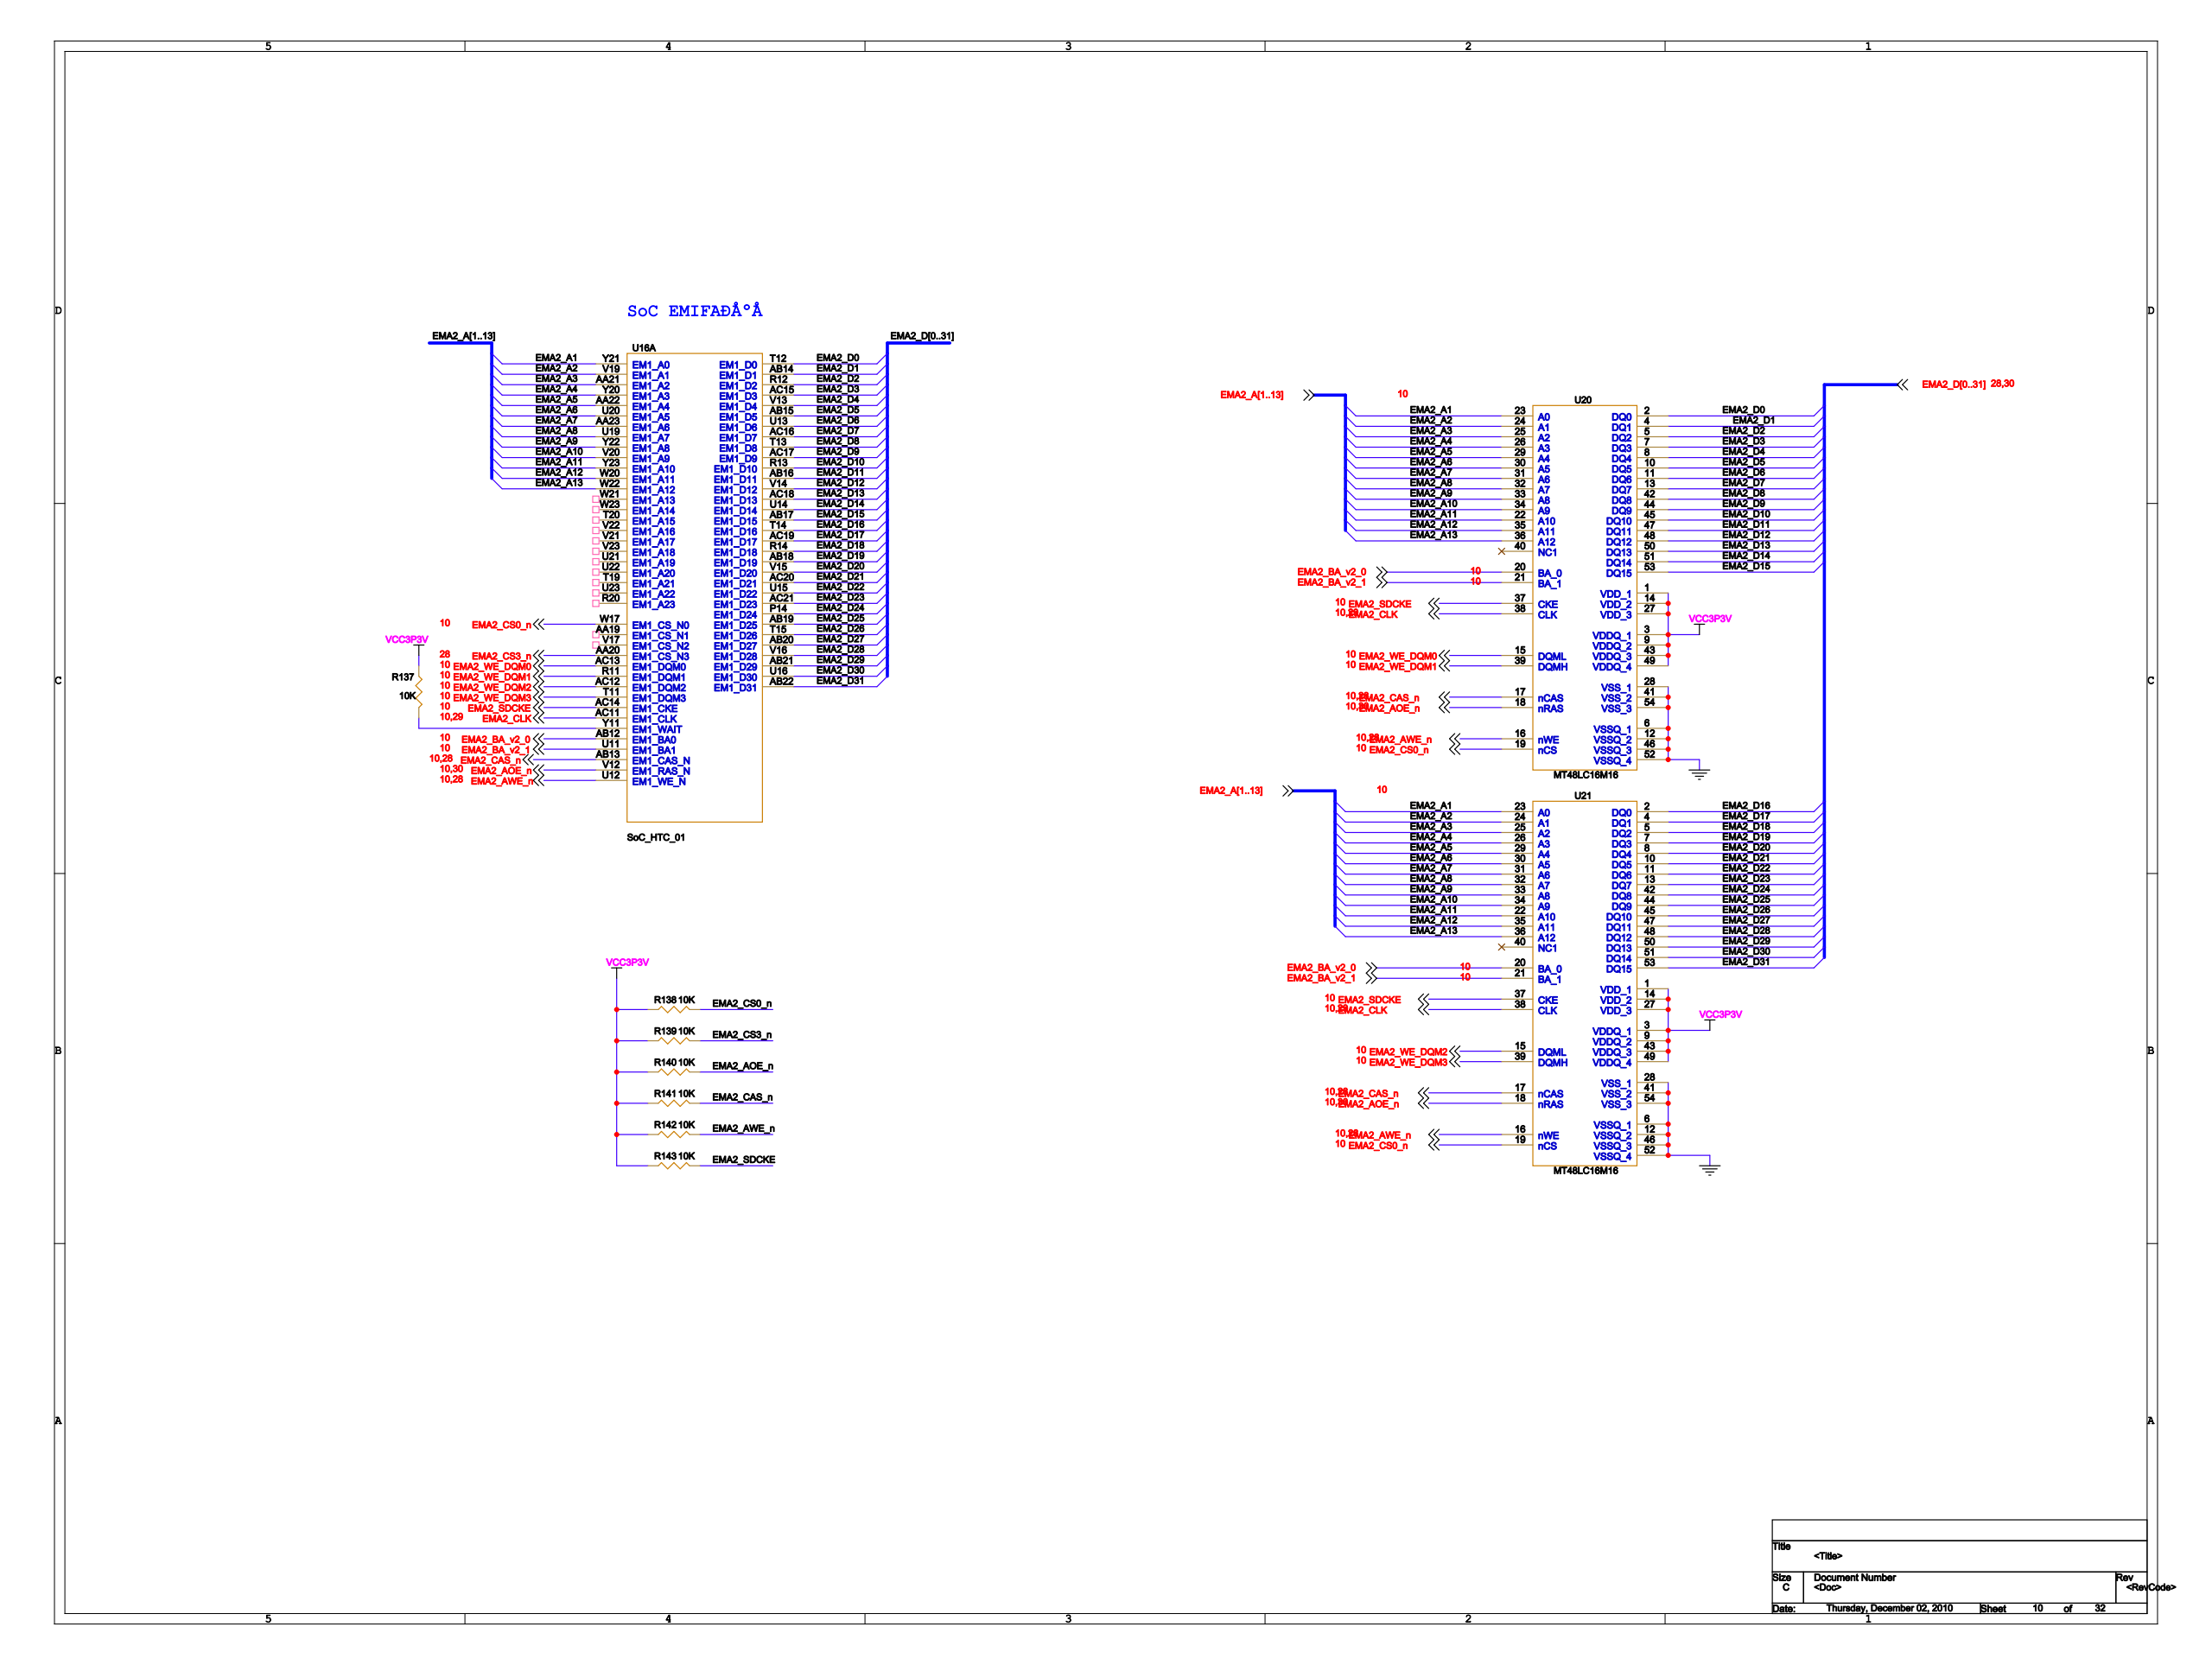Circuit board | Cadence Allegro | 1001 parts | 1318 nets | one sheet of the schematic
Parts on this sheet (reference | value | footprint):
R137 | 10K | 0603
R138 | 10K | 0603
R139 | 10K | 0603
R140 | 10K | 0603
R141 | 10K | 0603
R142 | 10K | 0603
R143 | 10K | 0603
U11 | MT48LC32M16 | TSOP54
U14 | MT48LC16M16 | TSOP54
U15 | MT48LC16M16 | TSOP54
U16 | SoC_HTC_01 | L529_XIN
U20 | MT48LC16M16 | TSOP54
U21 | MT48LC16M16 | TSOP54
U23 | MT48LC32M16 | TSOP54
Nets of these parts (net: part-pin ...):
EMA2_D11: U16-AB16 U20-47
EMA2_D3: U16-AC15 U20-7
EMA2_D7: U16-AC16 U20-13
EMA2_D15: U16-AB17 U20-53
EMA2_D27: U16-AB20 U21-47
EMA2_D23: U16-AC21 U21-13
EMA2_D29: U16-AB21 U21-50
EMA2_D31: U16-AB22 U21-53
EMA2_D9: U16-AC17 U20-44
EMA2_D12: U16-V14 U20-48
EMA2_AOE_N: R140-2 U16-V12 U20-18 U21-18
EMA2_D17: U16-AC19 U21-4
EMA2_D13: U16-AC18 U20-50
EMA2_D25: U16-AB19 U21-44
EMA2_D4: U16-V13 U20-8
EMA2_AWE_N: R142-2 U16-U12 U20-16 U21-16
EMA2_D6: U16-U13 U20-11
EMA2_CAS_N: R141-2 U16-AB13 U20-17 U21-17
EMA2_D5: U16-AB15 U20-10
EMA2_D22: U16-U15 U21-11
EMA2_D28: U16-V16 U21-48
EMA2_D21: U16-AC20 U21-10
EMA2_D1: U16-AB14 U20-4
EMA2_D2: U16-R12 U20-5
EMA2_D20: U16-V15 U21-8
EMA2_CS3_N: R139-2 U16-AA20
EMA2_D0: U16-T12 U20-2
EMA2_D30: U16-U16 U21-51
EMA2_D8: U16-T13 U20-42
EMA2_CLK: U16-AC11 U20-38 U21-38
EMA2_D10: U16-R13 U20-45
EMA2_D24: U16-P14 U21-42
EMA2_D16: U16-T14 U21-2
EMA2_D14: U16-U14 U20-51
EMA2_D26: U16-T15 U21-45
EMA2_D18: U16-R14 U21-5
EMA2_D19: U16-AB18 U21-7
VCC3P3V: R137-2 R138-1 R139-1 R140-1 R141-1 R142-1 R143-1 U11-1 U11-3 U11-9 U11-14 U11-27 U11-43 U11-49 U14-1 U14-3 U14-9 U14-14 U14-27 U14-43 U14-49 U15-1 U15-3 U15-9 U15-14 U15-27 U15-43 U15-49 U20-1 U20-3 U20-9 U20-14 U20-27 U20-43 U20-49 U21-1 U21-3 U21-9 U21-14 U21-27 U21-43 U21-49 U23-1 U23-3 U23-9 U23-14 U23-27 U23-43 U23-49
EMA2_A1: U16-Y21 U20-23 U21-23
EMA2_A2: U16-V19 U20-24 U21-24
EMA2_A11: U16-Y23 U20-22 U21-22
EMA2_A12: U16-W20 U20-35 U21-35
EMA2_A13: U16-W22 U20-36 U21-36
EMA2_A3: U16-AA21 U20-25 U21-25
EMA2_A4: U16-Y20 U20-26 U21-26
EMA2_A5: U16-AA22 U20-29 U21-29
EMA2_A6: U16-U20 U20-30 U21-30
EMA2_A7: U16-AA23 U20-31 U21-31
EMA2_A8: U16-U19 U20-32 U21-32
EMA2_A9: U16-Y22 U20-33 U21-33
EMA2_A10: U16-V20 U20-34 U21-34
EMA2_SDCKE: R143-2 U16-AC14 U20-37 U21-37
EMA2_CS0_N: R138-2 U16-W17 U20-19 U21-19
EMA2_WE_DQM0: U16-AC13 U20-15
EMA2_WE_DQM1: U16-R11 U20-39
EMA2_WE_DQM2: U16-AC12 U21-15
EMA2_WE_DQM3: U16-T11 U21-39
N16782079: R137-1 U16-Y11